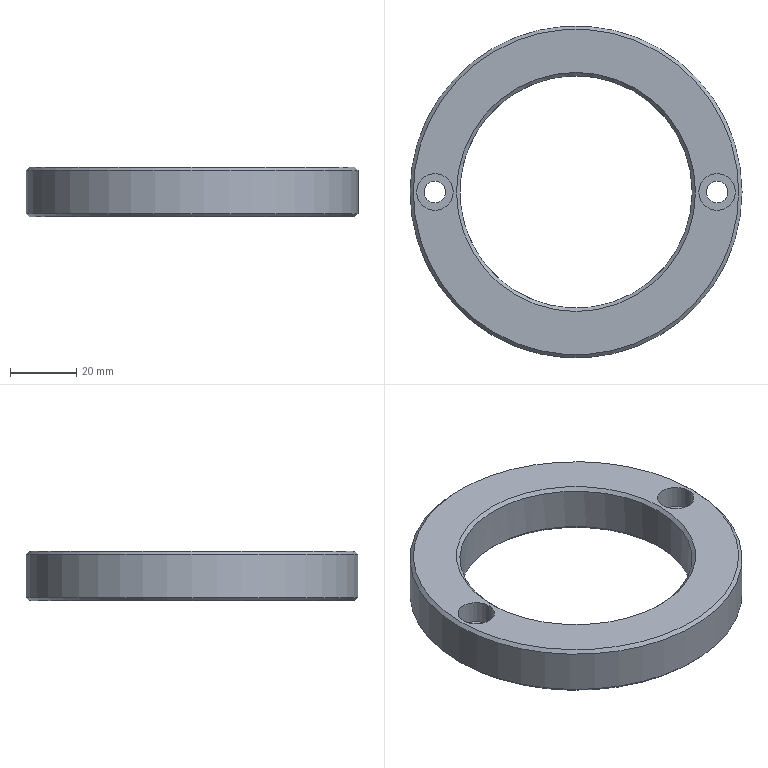Part | NX | features solid 2 | 1 solid | 14 faces | box 100 x 100 x 15 mm | volume 57687 mm3 | cylinder 6 | plane 4 | cone 4 | commonest cylinder face diameters 6.5 x2 11 x2 70 x1 100 x1
STEP:
#1=CARTESIAN_POINT('',(45.75,0.,95.5));
#2=VERTEX_POINT('',#1);
#3=CARTESIAN_POINT('',(42.5,0.,95.5));
#4=DIRECTION('',(0.,0.,1.));
#5=DIRECTION('',(1.,0.,0.));
#6=AXIS2_PLACEMENT_3D('',#3,#4,#5);
#7=CIRCLE('',#6,3.25);
#8=EDGE_CURVE('',#2,#2,#7,.T.);
#9=ORIENTED_EDGE('',*,*,#8,.T.);
#10=EDGE_LOOP('',(#9));
#11=FACE_BOUND('',#10,.T.);
#12=CARTESIAN_POINT('',(-36.,0.,95.5));
#13=VERTEX_POINT('',#12);
#14=CARTESIAN_POINT('',(0.,0.,95.5));
#15=DIRECTION('',(0.,0.,-1.));
#16=DIRECTION('',(-1.,0.,0.));
#17=AXIS2_PLACEMENT_3D('',#14,#15,#16);
#18=CIRCLE('',#17,36.);
#19=EDGE_CURVE('',#13,#13,#18,.F.);
#20=ORIENTED_EDGE('',*,*,#19,.T.);
#21=EDGE_LOOP('',(#20));
#22=FACE_BOUND('',#21,.T.);
#23=CARTESIAN_POINT('',(-49.,0.,95.5));
#24=VERTEX_POINT('',#23);
#25=CARTESIAN_POINT('',(0.,0.,95.5));
#26=DIRECTION('',(0.,0.,-1.));
#27=DIRECTION('',(-1.,0.,0.));
#28=AXIS2_PLACEMENT_3D('',#25,#26,#27);
#29=CIRCLE('',#28,49.);
#30=EDGE_CURVE('',#24,#24,#29,.T.);
#31=ORIENTED_EDGE('',*,*,#30,.T.);
#32=EDGE_LOOP('',(#31));
#33=FACE_BOUND('',#32,.T.);
#34=CARTESIAN_POINT('',(-39.25,0.,95.5));
#35=VERTEX_POINT('',#34);
#36=CARTESIAN_POINT('',(-42.5,0.,95.5));
#37=DIRECTION('',(0.,0.,1.));
#38=DIRECTION('',(1.,0.,0.));
#39=AXIS2_PLACEMENT_3D('',#36,#37,#38);
#40=CIRCLE('',#39,3.25);
#41=EDGE_CURVE('',#35,#35,#40,.T.);
#42=ORIENTED_EDGE('',*,*,#41,.T.);
#43=EDGE_LOOP('',(#42));
#44=FACE_BOUND('',#43,.T.);
#45=CARTESIAN_POINT('',(0.,0.,95.5));
#46=DIRECTION('',(0.,0.,-1.));
#47=DIRECTION('',(-1.,0.,0.));
#48=AXIS2_PLACEMENT_3D('',#45,#46,#47);
#49=PLANE('',#48);
#50=ADVANCED_FACE('',(#11,#22,#33,#44),#49,.T.);
#51=CARTESIAN_POINT('',(48.,0.,110.5));
#52=VERTEX_POINT('',#51);
#53=CARTESIAN_POINT('',(42.5,0.,110.5));
#54=DIRECTION('',(0.,0.,-1.));
#55=DIRECTION('',(1.,0.,0.));
#56=AXIS2_PLACEMENT_3D('',#53,#54,#55);
#57=CIRCLE('',#56,5.5);
#58=EDGE_CURVE('',#52,#52,#57,.T.);
#59=ORIENTED_EDGE('',*,*,#58,.T.);
#60=EDGE_LOOP('',(#59));
#61=FACE_BOUND('',#60,.T.);
#62=CARTESIAN_POINT('',(36.,0.,110.5));
#63=VERTEX_POINT('',#62);
#64=CARTESIAN_POINT('',(0.,0.,110.5));
#65=DIRECTION('',(0.,0.,1.));
#66=DIRECTION('',(1.,0.,0.));
#67=AXIS2_PLACEMENT_3D('',#64,#65,#66);
#68=CIRCLE('',#67,36.);
#69=EDGE_CURVE('',#63,#63,#68,.F.);
#70=ORIENTED_EDGE('',*,*,#69,.T.);
#71=EDGE_LOOP('',(#70));
#72=FACE_BOUND('',#71,.T.);
#73=CARTESIAN_POINT('',(49.,0.,110.5));
#74=VERTEX_POINT('',#73);
#75=CARTESIAN_POINT('',(0.,0.,110.5));
#76=DIRECTION('',(0.,0.,1.));
#77=DIRECTION('',(1.,0.,0.));
#78=AXIS2_PLACEMENT_3D('',#75,#76,#77);
#79=CIRCLE('',#78,49.);
#80=EDGE_CURVE('',#74,#74,#79,.T.);
#81=ORIENTED_EDGE('',*,*,#80,.T.);
#82=EDGE_LOOP('',(#81));
#83=FACE_BOUND('',#82,.T.);
#84=CARTESIAN_POINT('',(-37.,0.,110.5));
#85=VERTEX_POINT('',#84);
#86=CARTESIAN_POINT('',(-42.5,0.,110.5));
#87=DIRECTION('',(0.,0.,-1.));
#88=DIRECTION('',(1.,0.,0.));
#89=AXIS2_PLACEMENT_3D('',#86,#87,#88);
#90=CIRCLE('',#89,5.5);
#91=EDGE_CURVE('',#85,#85,#90,.T.);
#92=ORIENTED_EDGE('',*,*,#91,.T.);
#93=EDGE_LOOP('',(#92));
#94=FACE_BOUND('',#93,.T.);
#95=CARTESIAN_POINT('',(0.,0.,110.5));
#96=DIRECTION('',(0.,0.,1.));
#97=DIRECTION('',(1.,0.,0.));
#98=AXIS2_PLACEMENT_3D('',#95,#96,#97);
#99=PLANE('',#98);
#100=ADVANCED_FACE('',(#61,#72,#83,#94),#99,.T.);
#101=CARTESIAN_POINT('',(-50.,0.,96.5));
#102=VERTEX_POINT('',#101);
#103=CARTESIAN_POINT('',(0.,0.,96.5));
#104=DIRECTION('',(0.,0.,-1.));
#105=DIRECTION('',(-1.,0.,0.));
#106=AXIS2_PLACEMENT_3D('',#103,#104,#105);
#107=CIRCLE('',#106,50.);
#108=EDGE_CURVE('',#102,#102,#107,.F.);
#109=ORIENTED_EDGE('',*,*,#108,.T.);
#110=EDGE_LOOP('',(#109));
#111=FACE_BOUND('',#110,.T.);
#112=CARTESIAN_POINT('',(50.,0.,109.5));
#113=VERTEX_POINT('',#112);
#114=CARTESIAN_POINT('',(0.,0.,109.5));
#115=DIRECTION('',(0.,0.,1.));
#116=DIRECTION('',(1.,0.,0.));
#117=AXIS2_PLACEMENT_3D('',#114,#115,#116);
#118=CIRCLE('',#117,50.);
#119=EDGE_CURVE('',#113,#113,#118,.F.);
#120=ORIENTED_EDGE('',*,*,#119,.T.);
#121=EDGE_LOOP('',(#120));
#122=FACE_BOUND('',#121,.T.);
#123=CARTESIAN_POINT('',(0.,0.,95.5));
#124=DIRECTION('',(0.,0.,1.));
#125=DIRECTION('',(1.,0.,0.));
#126=AXIS2_PLACEMENT_3D('',#123,#124,#125);
#127=CYLINDRICAL_SURFACE('',#126,50.);
#128=ADVANCED_FACE('',(#111,#122),#127,.T.);
#129=CARTESIAN_POINT('',(-35.,0.,96.5));
#130=VERTEX_POINT('',#129);
#131=CARTESIAN_POINT('',(0.,0.,96.5));
#132=DIRECTION('',(0.,0.,-1.));
#133=DIRECTION('',(-1.,0.,0.));
#134=AXIS2_PLACEMENT_3D('',#131,#132,#133);
#135=CIRCLE('',#134,35.);
#136=EDGE_CURVE('',#130,#130,#135,.T.);
#137=ORIENTED_EDGE('',*,*,#136,.T.);
#138=EDGE_LOOP('',(#137));
#139=FACE_BOUND('',#138,.T.);
#140=CARTESIAN_POINT('',(35.,0.,109.5));
#141=VERTEX_POINT('',#140);
#142=CARTESIAN_POINT('',(0.,0.,109.5));
#143=DIRECTION('',(0.,0.,1.));
#144=DIRECTION('',(1.,0.,0.));
#145=AXIS2_PLACEMENT_3D('',#142,#143,#144);
#146=CIRCLE('',#145,35.);
#147=EDGE_CURVE('',#141,#141,#146,.T.);
#148=ORIENTED_EDGE('',*,*,#147,.T.);
#149=EDGE_LOOP('',(#148));
#150=FACE_BOUND('',#149,.T.);
#151=CARTESIAN_POINT('',(0.,0.,95.5));
#152=DIRECTION('',(0.,0.,1.));
#153=DIRECTION('',(1.,0.,0.));
#154=AXIS2_PLACEMENT_3D('',#151,#152,#153);
#155=CYLINDRICAL_SURFACE('',#154,35.);
#156=ADVANCED_FACE('',(#139,#150),#155,.F.);
#157=ORIENTED_EDGE('',*,*,#136,.F.);
#158=EDGE_LOOP('',(#157));
#159=FACE_BOUND('',#158,.T.);
#160=ORIENTED_EDGE('',*,*,#19,.F.);
#161=EDGE_LOOP('',(#160));
#162=FACE_BOUND('',#161,.T.);
#163=CARTESIAN_POINT('',(0.,0.,95.5));
#164=DIRECTION('',(0.,0.,-1.));
#165=DIRECTION('',(-1.,0.,0.));
#166=AXIS2_PLACEMENT_3D('',#163,#164,#165);
#167=CONICAL_SURFACE('',#166,36.,0.7854);
#168=ADVANCED_FACE('',(#159,#162),#167,.F.);
#169=ORIENTED_EDGE('',*,*,#147,.F.);
#170=EDGE_LOOP('',(#169));
#171=FACE_BOUND('',#170,.T.);
#172=ORIENTED_EDGE('',*,*,#69,.F.);
#173=EDGE_LOOP('',(#172));
#174=FACE_BOUND('',#173,.T.);
#175=CARTESIAN_POINT('',(0.,0.,110.5));
#176=DIRECTION('',(0.,0.,1.));
#177=DIRECTION('',(1.,0.,0.));
#178=AXIS2_PLACEMENT_3D('',#175,#176,#177);
#179=CONICAL_SURFACE('',#178,36.,0.7854);
#180=ADVANCED_FACE('',(#171,#174),#179,.F.);
#181=ORIENTED_EDGE('',*,*,#30,.F.);
#182=EDGE_LOOP('',(#181));
#183=FACE_BOUND('',#182,.T.);
#184=ORIENTED_EDGE('',*,*,#108,.F.);
#185=EDGE_LOOP('',(#184));
#186=FACE_BOUND('',#185,.T.);
#187=CARTESIAN_POINT('',(0.,0.,96.5));
#188=DIRECTION('',(0.,0.,1.));
#189=DIRECTION('',(1.,0.,0.));
#190=AXIS2_PLACEMENT_3D('',#187,#188,#189);
#191=CONICAL_SURFACE('',#190,50.,0.7854);
#192=ADVANCED_FACE('',(#183,#186),#191,.T.);
#193=ORIENTED_EDGE('',*,*,#80,.F.);
#194=EDGE_LOOP('',(#193));
#195=FACE_BOUND('',#194,.T.);
#196=ORIENTED_EDGE('',*,*,#119,.F.);
#197=EDGE_LOOP('',(#196));
#198=FACE_BOUND('',#197,.T.);
#199=CARTESIAN_POINT('',(0.,0.,109.5));
#200=DIRECTION('',(0.,0.,-1.));
#201=DIRECTION('',(-1.,0.,0.));
#202=AXIS2_PLACEMENT_3D('',#199,#200,#201);
#203=CONICAL_SURFACE('',#202,50.,0.7854);
#204=ADVANCED_FACE('',(#195,#198),#203,.T.);
#205=CARTESIAN_POINT('',(39.25,0.,103.5));
#206=VERTEX_POINT('',#205);
#207=CARTESIAN_POINT('',(42.5,0.,103.5));
#208=DIRECTION('',(0.,0.,-1.));
#209=DIRECTION('',(-1.,0.,0.));
#210=AXIS2_PLACEMENT_3D('',#207,#208,#209);
#211=CIRCLE('',#210,3.25);
#212=EDGE_CURVE('',#206,#206,#211,.T.);
#213=ORIENTED_EDGE('',*,*,#212,.T.);
#214=EDGE_LOOP('',(#213));
#215=FACE_BOUND('',#214,.T.);
#216=CARTESIAN_POINT('',(48.,0.,103.5));
#217=VERTEX_POINT('',#216);
#218=CARTESIAN_POINT('',(42.5,0.,103.5));
#219=DIRECTION('',(0.,0.,1.));
#220=DIRECTION('',(1.,0.,0.));
#221=AXIS2_PLACEMENT_3D('',#218,#219,#220);
#222=CIRCLE('',#221,5.5);
#223=EDGE_CURVE('',#217,#217,#222,.F.);
#224=ORIENTED_EDGE('',*,*,#223,.F.);
#225=EDGE_LOOP('',(#224));
#226=FACE_BOUND('',#225,.T.);
#227=CARTESIAN_POINT('',(42.5,0.,103.5));
#228=DIRECTION('',(0.,0.,-1.));
#229=DIRECTION('',(-1.,0.,0.));
#230=AXIS2_PLACEMENT_3D('',#227,#228,#229);
#231=PLANE('',#230);
#232=ADVANCED_FACE('',(#215,#226),#231,.F.);
#233=ORIENTED_EDGE('',*,*,#223,.T.);
#234=EDGE_LOOP('',(#233));
#235=FACE_BOUND('',#234,.T.);
#236=ORIENTED_EDGE('',*,*,#58,.F.);
#237=EDGE_LOOP('',(#236));
#238=FACE_BOUND('',#237,.T.);
#239=CARTESIAN_POINT('',(42.5,0.,110.5));
#240=DIRECTION('',(0.,0.,-1.));
#241=DIRECTION('',(1.,0.,0.));
#242=AXIS2_PLACEMENT_3D('',#239,#240,#241);
#243=CYLINDRICAL_SURFACE('',#242,5.5);
#244=ADVANCED_FACE('',(#235,#238),#243,.F.);
#245=ORIENTED_EDGE('',*,*,#8,.F.);
#246=EDGE_LOOP('',(#245));
#247=FACE_BOUND('',#246,.T.);
#248=ORIENTED_EDGE('',*,*,#212,.F.);
#249=EDGE_LOOP('',(#248));
#250=FACE_BOUND('',#249,.T.);
#251=CARTESIAN_POINT('',(42.5,0.,110.5));
#252=DIRECTION('',(0.,0.,-1.));
#253=DIRECTION('',(1.,0.,0.));
#254=AXIS2_PLACEMENT_3D('',#251,#252,#253);
#255=CYLINDRICAL_SURFACE('',#254,3.25);
#256=ADVANCED_FACE('',(#247,#250),#255,.F.);
#257=CARTESIAN_POINT('',(-45.75,0.,103.5));
#258=VERTEX_POINT('',#257);
#259=CARTESIAN_POINT('',(-42.5,0.,103.5));
#260=DIRECTION('',(0.,0.,-1.));
#261=DIRECTION('',(-1.,0.,0.));
#262=AXIS2_PLACEMENT_3D('',#259,#260,#261);
#263=CIRCLE('',#262,3.25);
#264=EDGE_CURVE('',#258,#258,#263,.T.);
#265=ORIENTED_EDGE('',*,*,#264,.T.);
#266=EDGE_LOOP('',(#265));
#267=FACE_BOUND('',#266,.T.);
#268=CARTESIAN_POINT('',(-37.,0.,103.5));
#269=VERTEX_POINT('',#268);
#270=CARTESIAN_POINT('',(-42.5,0.,103.5));
#271=DIRECTION('',(0.,0.,1.));
#272=DIRECTION('',(1.,0.,0.));
#273=AXIS2_PLACEMENT_3D('',#270,#271,#272);
#274=CIRCLE('',#273,5.5);
#275=EDGE_CURVE('',#269,#269,#274,.F.);
#276=ORIENTED_EDGE('',*,*,#275,.F.);
#277=EDGE_LOOP('',(#276));
#278=FACE_BOUND('',#277,.T.);
#279=CARTESIAN_POINT('',(-42.5,0.,103.5));
#280=DIRECTION('',(0.,0.,-1.));
#281=DIRECTION('',(-1.,0.,0.));
#282=AXIS2_PLACEMENT_3D('',#279,#280,#281);
#283=PLANE('',#282);
#284=ADVANCED_FACE('',(#267,#278),#283,.F.);
#285=ORIENTED_EDGE('',*,*,#275,.T.);
#286=EDGE_LOOP('',(#285));
#287=FACE_BOUND('',#286,.T.);
#288=ORIENTED_EDGE('',*,*,#91,.F.);
#289=EDGE_LOOP('',(#288));
#290=FACE_BOUND('',#289,.T.);
#291=CARTESIAN_POINT('',(-42.5,0.,110.5));
#292=DIRECTION('',(0.,0.,-1.));
#293=DIRECTION('',(1.,0.,0.));
#294=AXIS2_PLACEMENT_3D('',#291,#292,#293);
#295=CYLINDRICAL_SURFACE('',#294,5.5);
#296=ADVANCED_FACE('',(#287,#290),#295,.F.);
#297=ORIENTED_EDGE('',*,*,#41,.F.);
#298=EDGE_LOOP('',(#297));
#299=FACE_BOUND('',#298,.T.);
#300=ORIENTED_EDGE('',*,*,#264,.F.);
#301=EDGE_LOOP('',(#300));
#302=FACE_BOUND('',#301,.T.);
#303=CARTESIAN_POINT('',(-42.5,0.,110.5));
#304=DIRECTION('',(0.,0.,-1.));
#305=DIRECTION('',(1.,0.,0.));
#306=AXIS2_PLACEMENT_3D('',#303,#304,#305);
#307=CYLINDRICAL_SURFACE('',#306,3.25);
#308=ADVANCED_FACE('',(#299,#302),#307,.F.);
#309=CLOSED_SHELL('',(#50,#100,#128,#156,#168,#180,#192,#204,#232,#244,#256,#284,#296,#308));
#310=MANIFOLD_SOLID_BREP('',#309);
#311=(LENGTH_UNIT()NAMED_UNIT(*)SI_UNIT(.MILLI.,.METRE.));
#312=UNCERTAINTY_MEASURE_WITH_UNIT(LENGTH_MEASURE(0.00001),#311,'','');
#313=(NAMED_UNIT(*)PLANE_ANGLE_UNIT()SI_UNIT($,.RADIAN.));
#314=(NAMED_UNIT(*)SI_UNIT($,.STERADIAN.)SOLID_ANGLE_UNIT());
#315=(GEOMETRIC_REPRESENTATION_CONTEXT(3)GLOBAL_UNCERTAINTY_ASSIGNED_CONTEXT((#312))GLOBAL_UNIT_ASSIGNED_CONTEXT((#311,#313,#314))REPRESENTATION_CONTEXT('',''));
#316=ADVANCED_BREP_SHAPE_REPRESENTATION('',(#310),#315);